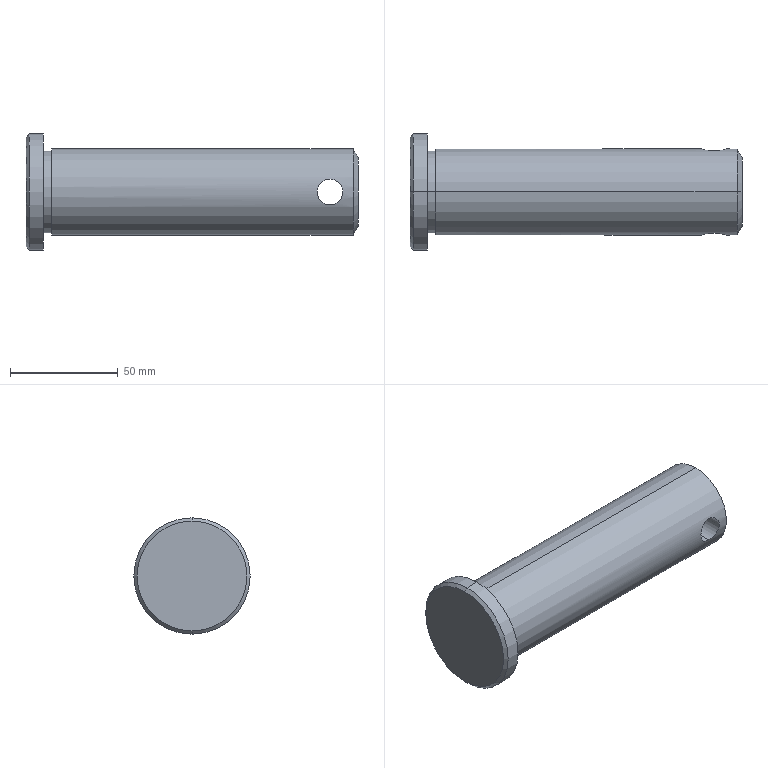Part | SolidWorks | features Chamfer 2, ICE 1, Revolution 1 | 1 solid | 16 faces | box 154 x 54 x 54 mm | volume 196099 mm3 | cylinder 8 | cone 4 | plane 4 | commonest cylinder face diameters 12 x2 38 x2 40 x2 54 x2
STEP:
#1=CARTESIAN_POINT('',(141.,-19.079,-6.));
#2=VERTEX_POINT('',#1);
#3=CARTESIAN_POINT('',(141.,-19.079,6.));
#4=VERTEX_POINT('',#3);
#5=CARTESIAN_POINT('',(141.,-19.079,-6.));
#6=CARTESIAN_POINT('',(140.607,-19.079,-6.));
#7=CARTESIAN_POINT('',(140.213,-19.091,-5.961));
#8=CARTESIAN_POINT('',(139.434,-19.139,-5.806));
#9=CARTESIAN_POINT('',(139.059,-19.174,-5.691));
#10=CARTESIAN_POINT('',(138.336,-19.261,-5.39));
#11=CARTESIAN_POINT('',(137.985,-19.313,-5.202));
#12=CARTESIAN_POINT('',(137.336,-19.425,-4.767));
#13=CARTESIAN_POINT('',(137.035,-19.484,-4.521));
#14=CARTESIAN_POINT('',(136.62,-19.575,-4.105));
#15=CARTESIAN_POINT('',(136.487,-19.605,-3.959));
#16=CARTESIAN_POINT('',(136.239,-19.664,-3.657));
#17=CARTESIAN_POINT('',(136.123,-19.692,-3.5));
#18=CARTESIAN_POINT('',(135.798,-19.774,-3.015));
#19=CARTESIAN_POINT('',(135.612,-19.824,-2.67));
#20=CARTESIAN_POINT('',(135.308,-19.909,-1.939));
#21=CARTESIAN_POINT('',(135.194,-19.943,-1.564));
#22=CARTESIAN_POINT('',(135.078,-19.977,-0.9868));
#23=CARTESIAN_POINT('',(135.049,-19.985,-0.7922));
#24=CARTESIAN_POINT('',(135.01,-19.997,-0.398));
#25=CARTESIAN_POINT('',(135.,-20.,-0.1981));
#26=CARTESIAN_POINT('',(135.,-20.,0.3951));
#27=CARTESIAN_POINT('',(135.039,-19.988,0.7861));
#28=CARTESIAN_POINT('',(135.154,-19.954,1.366));
#29=CARTESIAN_POINT('',(135.203,-19.94,1.559));
#30=CARTESIAN_POINT('',(135.318,-19.907,1.938));
#31=CARTESIAN_POINT('',(135.385,-19.888,2.123));
#32=CARTESIAN_POINT('',(135.61,-19.825,2.665));
#33=CARTESIAN_POINT('',(135.795,-19.775,3.01));
#34=CARTESIAN_POINT('',(136.234,-19.664,3.666));
#35=CARTESIAN_POINT('',(136.481,-19.605,3.967));
#36=CARTESIAN_POINT('',(136.894,-19.515,4.379));
#37=CARTESIAN_POINT('',(137.038,-19.485,4.51));
#38=CARTESIAN_POINT('',(137.341,-19.426,4.759));
#39=CARTESIAN_POINT('',(137.5,-19.397,4.877));
#40=CARTESIAN_POINT('',(137.988,-19.312,5.204));
#41=CARTESIAN_POINT('',(138.331,-19.261,5.388));
#42=CARTESIAN_POINT('',(139.054,-19.174,5.689));
#43=CARTESIAN_POINT('',(139.437,-19.139,5.806));
#44=CARTESIAN_POINT('',(140.209,-19.091,5.961));
#45=CARTESIAN_POINT('',(140.601,-19.079,6.));
#46=CARTESIAN_POINT('',(141.,-19.079,6.));
#47=B_SPLINE_CURVE_WITH_KNOTS('',3,(#5,#6,#7,#8,#9,#10,#11,#12,#13,#14,#15,#16,#17,#18,#19,#20,#21,#22,#23,#24,#25,#26,#27,#28,#29,#30,#31,#32,#33,#34,#35,#36,#37,#38,#39,#40,#41,#42,#43,#44,#45,#46),.UNSPECIFIED.,.F.,.F.,(4,2,2,2,2,2,2,2,2,2,2,2,2,2,2,2,2,2,2,2,4),(0.01887,0.02005,0.02123,0.0224,0.02358,0.02417,0.02476,0.02594,0.02712,0.02771,0.0283,0.02948,0.03007,0.03066,0.03184,0.03301,0.0336,0.03419,0.03537,0.03655,0.03773),.UNSPECIFIED.);
#48=EDGE_CURVE('',#2,#4,#47,.T.);
#49=ORIENTED_EDGE('',*,*,#48,.F.);
#50=CARTESIAN_POINT('',(141.,19.079,-6.));
#51=VERTEX_POINT('',#50);
#52=CARTESIAN_POINT('',(141.,-27.,-6.));
#53=DIRECTION('',(0.,1.,0.));
#54=VECTOR('',#53,1000.);
#55=LINE('',#52,#54);
#56=EDGE_CURVE('',#2,#51,#55,.T.);
#57=ORIENTED_EDGE('',*,*,#56,.T.);
#58=CARTESIAN_POINT('',(141.,19.079,6.));
#59=VERTEX_POINT('',#58);
#60=CARTESIAN_POINT('',(141.,19.079,6.));
#61=CARTESIAN_POINT('',(140.601,19.079,6.));
#62=CARTESIAN_POINT('',(140.209,19.091,5.961));
#63=CARTESIAN_POINT('',(139.632,19.127,5.845));
#64=CARTESIAN_POINT('',(139.441,19.141,5.797));
#65=CARTESIAN_POINT('',(139.063,19.176,5.682));
#66=CARTESIAN_POINT('',(138.876,19.196,5.615));
#67=CARTESIAN_POINT('',(138.332,19.261,5.388));
#68=CARTESIAN_POINT('',(137.988,19.312,5.204));
#69=CARTESIAN_POINT('',(137.5,19.396,4.877));
#70=CARTESIAN_POINT('',(137.341,19.426,4.759));
#71=CARTESIAN_POINT('',(137.038,19.485,4.51));
#72=CARTESIAN_POINT('',(136.894,19.515,4.379));
#73=CARTESIAN_POINT('',(136.482,19.605,3.967));
#74=CARTESIAN_POINT('',(136.234,19.664,3.666));
#75=CARTESIAN_POINT('',(135.795,19.775,3.011));
#76=CARTESIAN_POINT('',(135.61,19.825,2.665));
#77=CARTESIAN_POINT('',(135.385,19.888,2.124));
#78=CARTESIAN_POINT('',(135.319,19.907,1.94));
#79=CARTESIAN_POINT('',(135.204,19.94,1.563));
#80=CARTESIAN_POINT('',(135.155,19.954,1.369));
#81=CARTESIAN_POINT('',(135.039,19.988,0.7875));
#82=CARTESIAN_POINT('',(135.,20.,0.3966));
#83=CARTESIAN_POINT('',(135.,20.,-0.3914));
#84=CARTESIAN_POINT('',(135.039,19.988,-0.7916));
#85=CARTESIAN_POINT('',(135.194,19.943,-1.563));
#86=CARTESIAN_POINT('',(135.308,19.909,-1.938));
#87=CARTESIAN_POINT('',(135.611,19.825,-2.668));
#88=CARTESIAN_POINT('',(135.798,19.774,-3.015));
#89=CARTESIAN_POINT('',(136.123,19.692,-3.501));
#90=CARTESIAN_POINT('',(136.24,19.663,-3.657));
#91=CARTESIAN_POINT('',(136.488,19.605,-3.96));
#92=CARTESIAN_POINT('',(136.621,19.574,-4.106));
#93=CARTESIAN_POINT('',(137.037,19.484,-4.522));
#94=CARTESIAN_POINT('',(137.337,19.425,-4.768));
#95=CARTESIAN_POINT('',(137.985,19.313,-5.202));
#96=CARTESIAN_POINT('',(138.337,19.26,-5.391));
#97=CARTESIAN_POINT('',(139.06,19.174,-5.691));
#98=CARTESIAN_POINT('',(139.434,19.139,-5.805));
#99=CARTESIAN_POINT('',(140.015,19.103,-5.922));
#100=CARTESIAN_POINT('',(140.213,19.094,-5.951));
#101=CARTESIAN_POINT('',(140.607,19.082,-5.99));
#102=CARTESIAN_POINT('',(140.803,19.079,-6.));
#103=CARTESIAN_POINT('',(141.,19.079,-6.));
#104=B_SPLINE_CURVE_WITH_KNOTS('',3,(#60,#61,#62,#63,#64,#65,#66,#67,#68,#69,#70,#71,#72,#73,#74,#75,#76,#77,#78,#79,#80,#81,#82,#83,#84,#85,#86,#87,#88,#89,#90,#91,#92,#93,#94,#95,#96,#97,#98,#99,#100,#101,#102,#103),.UNSPECIFIED.,.F.,.F.,(4,2,2,2,2,2,2,2,2,2,2,2,2,2,2,2,2,2,2,2,2,4),(0.,0.001179,0.001769,0.002358,0.003538,0.004127,0.004717,0.005896,0.007075,0.007665,0.008255,0.009434,0.01061,0.01179,0.01297,0.01356,0.01415,0.01533,0.01651,0.01769,0.01828,0.01887),.UNSPECIFIED.);
#105=EDGE_CURVE('',#59,#51,#104,.T.);
#106=ORIENTED_EDGE('',*,*,#105,.F.);
#107=CARTESIAN_POINT('',(141.,-27.,6.));
#108=DIRECTION('',(0.,1.,0.));
#109=VECTOR('',#108,1000.);
#110=LINE('',#107,#109);
#111=EDGE_CURVE('',#4,#59,#110,.T.);
#112=ORIENTED_EDGE('',*,*,#111,.F.);
#113=EDGE_LOOP('',(#49,#57,#106,#112));
#114=FACE_OUTER_BOUND('',#113,.T.);
#115=CARTESIAN_POINT('',(141.,-27.,0.));
#116=DIRECTION('',(0.,1.,0.));
#117=DIRECTION('',(0.,0.,1.));
#118=AXIS2_PLACEMENT_3D('',#115,#116,#117);
#119=CYLINDRICAL_SURFACE('',#118,6.);
#120=ADVANCED_FACE('',(#114),#119,.F.);
#121=CARTESIAN_POINT('',(154.,0.,-16.));
#122=VERTEX_POINT('',#121);
#123=CARTESIAN_POINT('',(154.,0.,16.));
#124=VERTEX_POINT('',#123);
#125=CARTESIAN_POINT('',(154.,0.,0.));
#126=DIRECTION('',(1.,0.,0.));
#127=DIRECTION('',(0.,0.,1.));
#128=AXIS2_PLACEMENT_3D('',#125,#126,#127);
#129=CIRCLE('',#128,16.);
#130=EDGE_CURVE('',#122,#124,#129,.T.);
#131=ORIENTED_EDGE('',*,*,#130,.F.);
#132=CARTESIAN_POINT('',(151.691,0.,-20.));
#133=VERTEX_POINT('',#132);
#134=CARTESIAN_POINT('',(151.691,0.,-20.));
#135=DIRECTION('',(-0.5,0.,-0.866));
#136=VECTOR('',#135,1000.);
#137=LINE('',#134,#136);
#138=EDGE_CURVE('',#122,#133,#137,.T.);
#139=ORIENTED_EDGE('',*,*,#138,.T.);
#140=CARTESIAN_POINT('',(151.691,0.,20.));
#141=VERTEX_POINT('',#140);
#142=CARTESIAN_POINT('',(151.691,0.,0.));
#143=DIRECTION('',(-1.,0.,0.));
#144=DIRECTION('',(0.,0.,1.));
#145=AXIS2_PLACEMENT_3D('',#142,#143,#144);
#146=CIRCLE('',#145,20.);
#147=EDGE_CURVE('',#141,#133,#146,.T.);
#148=ORIENTED_EDGE('',*,*,#147,.F.);
#149=CARTESIAN_POINT('',(151.691,0.,20.));
#150=DIRECTION('',(-0.5,0.,0.866));
#151=VECTOR('',#150,1000.);
#152=LINE('',#149,#151);
#153=EDGE_CURVE('',#124,#141,#152,.T.);
#154=ORIENTED_EDGE('',*,*,#153,.F.);
#155=EDGE_LOOP('',(#131,#139,#148,#154));
#156=FACE_OUTER_BOUND('',#155,.T.);
#157=CARTESIAN_POINT('',(151.691,0.,0.));
#158=DIRECTION('',(-1.,0.,0.));
#159=DIRECTION('',(0.,0.,1.));
#160=AXIS2_PLACEMENT_3D('',#157,#158,#159);
#161=CONICAL_SURFACE('',#160,20.,1.047);
#162=ADVANCED_FACE('',(#156),#161,.T.);
#163=CARTESIAN_POINT('',(0.,0.,25.5));
#164=VERTEX_POINT('',#163);
#165=CARTESIAN_POINT('',(0.,0.,-25.5));
#166=VERTEX_POINT('',#165);
#167=CARTESIAN_POINT('',(0.,0.,0.));
#168=DIRECTION('',(-1.,0.,0.));
#169=DIRECTION('',(0.,0.,-1.));
#170=AXIS2_PLACEMENT_3D('',#167,#168,#169);
#171=CIRCLE('',#170,25.5);
#172=EDGE_CURVE('',#164,#166,#171,.T.);
#173=ORIENTED_EDGE('',*,*,#172,.F.);
#174=CARTESIAN_POINT('',(1.5,0.,27.));
#175=VERTEX_POINT('',#174);
#176=CARTESIAN_POINT('',(0.,0.,25.5));
#177=DIRECTION('',(0.7071,0.,0.7071));
#178=VECTOR('',#177,1000.);
#179=LINE('',#176,#178);
#180=EDGE_CURVE('',#164,#175,#179,.T.);
#181=ORIENTED_EDGE('',*,*,#180,.T.);
#182=CARTESIAN_POINT('',(1.5,0.,-27.));
#183=VERTEX_POINT('',#182);
#184=CARTESIAN_POINT('',(1.5,0.,0.));
#185=DIRECTION('',(1.,0.,0.));
#186=DIRECTION('',(0.,0.,-1.));
#187=AXIS2_PLACEMENT_3D('',#184,#185,#186);
#188=CIRCLE('',#187,27.);
#189=EDGE_CURVE('',#183,#175,#188,.T.);
#190=ORIENTED_EDGE('',*,*,#189,.F.);
#191=CARTESIAN_POINT('',(0.,0.,-25.5));
#192=DIRECTION('',(0.7071,0.,-0.7071));
#193=VECTOR('',#192,1000.);
#194=LINE('',#191,#193);
#195=EDGE_CURVE('',#166,#183,#194,.T.);
#196=ORIENTED_EDGE('',*,*,#195,.F.);
#197=EDGE_LOOP('',(#173,#181,#190,#196));
#198=FACE_OUTER_BOUND('',#197,.T.);
#199=CARTESIAN_POINT('',(0.,0.,0.));
#200=DIRECTION('',(1.,0.,0.));
#201=DIRECTION('',(0.,0.,-1.));
#202=AXIS2_PLACEMENT_3D('',#199,#200,#201);
#203=CONICAL_SURFACE('',#202,25.5,0.7854);
#204=ADVANCED_FACE('',(#198),#203,.T.);
#205=CARTESIAN_POINT('',(8.,0.,27.));
#206=VERTEX_POINT('',#205);
#207=CARTESIAN_POINT('',(8.,0.,-27.));
#208=VERTEX_POINT('',#207);
#209=CARTESIAN_POINT('',(8.,0.,0.));
#210=DIRECTION('',(-1.,0.,0.));
#211=DIRECTION('',(0.,0.,1.));
#212=AXIS2_PLACEMENT_3D('',#209,#210,#211);
#213=CIRCLE('',#212,27.);
#214=EDGE_CURVE('',#206,#208,#213,.T.);
#215=ORIENTED_EDGE('',*,*,#214,.T.);
#216=CARTESIAN_POINT('',(-105.652,0.,-27.));
#217=DIRECTION('',(-1.,0.,0.));
#218=VECTOR('',#217,1000.);
#219=LINE('',#216,#218);
#220=EDGE_CURVE('',#208,#183,#219,.T.);
#221=ORIENTED_EDGE('',*,*,#220,.T.);
#222=ORIENTED_EDGE('',*,*,#189,.T.);
#223=CARTESIAN_POINT('',(-105.652,0.,27.));
#224=DIRECTION('',(-1.,0.,0.));
#225=VECTOR('',#224,1000.);
#226=LINE('',#223,#225);
#227=EDGE_CURVE('',#206,#175,#226,.T.);
#228=ORIENTED_EDGE('',*,*,#227,.F.);
#229=EDGE_LOOP('',(#215,#221,#222,#228));
#230=FACE_OUTER_BOUND('',#229,.T.);
#231=CARTESIAN_POINT('',(-105.652,0.,0.));
#232=DIRECTION('',(-1.,0.,0.));
#233=DIRECTION('',(0.,0.,1.));
#234=AXIS2_PLACEMENT_3D('',#231,#232,#233);
#235=CYLINDRICAL_SURFACE('',#234,27.);
#236=ADVANCED_FACE('',(#230),#235,.T.);
#237=CARTESIAN_POINT('',(12.,0.,19.));
#238=VERTEX_POINT('',#237);
#239=CARTESIAN_POINT('',(12.,0.,-19.));
#240=VERTEX_POINT('',#239);
#241=CARTESIAN_POINT('',(12.,0.,0.));
#242=DIRECTION('',(-1.,0.,0.));
#243=DIRECTION('',(0.,0.,1.));
#244=AXIS2_PLACEMENT_3D('',#241,#242,#243);
#245=CIRCLE('',#244,19.);
#246=EDGE_CURVE('',#238,#240,#245,.T.);
#247=ORIENTED_EDGE('',*,*,#246,.T.);
#248=CARTESIAN_POINT('',(8.,0.,-19.));
#249=VERTEX_POINT('',#248);
#250=CARTESIAN_POINT('',(-105.652,0.,-19.));
#251=DIRECTION('',(-1.,0.,0.));
#252=VECTOR('',#251,1000.);
#253=LINE('',#250,#252);
#254=EDGE_CURVE('',#240,#249,#253,.T.);
#255=ORIENTED_EDGE('',*,*,#254,.T.);
#256=CARTESIAN_POINT('',(8.,0.,19.));
#257=VERTEX_POINT('',#256);
#258=CARTESIAN_POINT('',(8.,0.,0.));
#259=DIRECTION('',(-1.,0.,0.));
#260=DIRECTION('',(0.,0.,1.));
#261=AXIS2_PLACEMENT_3D('',#258,#259,#260);
#262=CIRCLE('',#261,19.);
#263=EDGE_CURVE('',#257,#249,#262,.T.);
#264=ORIENTED_EDGE('',*,*,#263,.F.);
#265=CARTESIAN_POINT('',(-105.652,0.,19.));
#266=DIRECTION('',(-1.,0.,0.));
#267=VECTOR('',#266,1000.);
#268=LINE('',#265,#267);
#269=EDGE_CURVE('',#238,#257,#268,.T.);
#270=ORIENTED_EDGE('',*,*,#269,.F.);
#271=EDGE_LOOP('',(#247,#255,#264,#270));
#272=FACE_OUTER_BOUND('',#271,.T.);
#273=CARTESIAN_POINT('',(-105.652,0.,0.));
#274=DIRECTION('',(-1.,0.,0.));
#275=DIRECTION('',(0.,0.,1.));
#276=AXIS2_PLACEMENT_3D('',#273,#274,#275);
#277=CYLINDRICAL_SURFACE('',#276,19.);
#278=ADVANCED_FACE('',(#272),#277,.T.);
#279=ORIENTED_EDGE('',*,*,#105,.T.);
#280=CARTESIAN_POINT('',(141.,19.079,-6.));
#281=CARTESIAN_POINT('',(141.393,19.079,-6.));
#282=CARTESIAN_POINT('',(141.787,19.091,-5.961));
#283=CARTESIAN_POINT('',(142.566,19.139,-5.806));
#284=CARTESIAN_POINT('',(142.941,19.174,-5.691));
#285=CARTESIAN_POINT('',(143.664,19.261,-5.39));
#286=CARTESIAN_POINT('',(144.015,19.313,-5.202));
#287=CARTESIAN_POINT('',(144.664,19.425,-4.767));
#288=CARTESIAN_POINT('',(144.965,19.484,-4.521));
#289=CARTESIAN_POINT('',(145.38,19.575,-4.105));
#290=CARTESIAN_POINT('',(145.513,19.605,-3.959));
#291=CARTESIAN_POINT('',(145.761,19.664,-3.657));
#292=CARTESIAN_POINT('',(145.877,19.692,-3.5));
#293=CARTESIAN_POINT('',(146.202,19.774,-3.015));
#294=CARTESIAN_POINT('',(146.388,19.824,-2.67));
#295=CARTESIAN_POINT('',(146.692,19.909,-1.939));
#296=CARTESIAN_POINT('',(146.806,19.943,-1.564));
#297=CARTESIAN_POINT('',(146.922,19.977,-0.9868));
#298=CARTESIAN_POINT('',(146.951,19.985,-0.7922));
#299=CARTESIAN_POINT('',(146.99,19.997,-0.398));
#300=CARTESIAN_POINT('',(147.,20.,-0.1981));
#301=CARTESIAN_POINT('',(147.,20.,0.3951));
#302=CARTESIAN_POINT('',(146.961,19.988,0.7861));
#303=CARTESIAN_POINT('',(146.846,19.954,1.366));
#304=CARTESIAN_POINT('',(146.797,19.94,1.559));
#305=CARTESIAN_POINT('',(146.682,19.907,1.938));
#306=CARTESIAN_POINT('',(146.615,19.888,2.123));
#307=CARTESIAN_POINT('',(146.39,19.825,2.665));
#308=CARTESIAN_POINT('',(146.205,19.775,3.01));
#309=CARTESIAN_POINT('',(145.766,19.664,3.666));
#310=CARTESIAN_POINT('',(145.519,19.605,3.967));
#311=CARTESIAN_POINT('',(145.106,19.515,4.379));
#312=CARTESIAN_POINT('',(144.962,19.485,4.51));
#313=CARTESIAN_POINT('',(144.659,19.426,4.759));
#314=CARTESIAN_POINT('',(144.5,19.397,4.877));
#315=CARTESIAN_POINT('',(144.012,19.312,5.204));
#316=CARTESIAN_POINT('',(143.669,19.261,5.388));
#317=CARTESIAN_POINT('',(142.946,19.174,5.689));
#318=CARTESIAN_POINT('',(142.563,19.139,5.806));
#319=CARTESIAN_POINT('',(141.791,19.091,5.961));
#320=CARTESIAN_POINT('',(141.399,19.079,6.));
#321=CARTESIAN_POINT('',(141.,19.079,6.));
#322=B_SPLINE_CURVE_WITH_KNOTS('',3,(#280,#281,#282,#283,#284,#285,#286,#287,#288,#289,#290,#291,#292,#293,#294,#295,#296,#297,#298,#299,#300,#301,#302,#303,#304,#305,#306,#307,#308,#309,#310,#311,#312,#313,#314,#315,#316,#317,#318,#319,#320,#321),.UNSPECIFIED.,.F.,.F.,(4,2,2,2,2,2,2,2,2,2,2,2,2,2,2,2,2,2,2,2,4),(0.01887,0.02005,0.02123,0.0224,0.02358,0.02417,0.02476,0.02594,0.02712,0.02771,0.0283,0.02948,0.03007,0.03066,0.03184,0.03301,0.0336,0.03419,0.03537,0.03655,0.03773),.UNSPECIFIED.);
#323=EDGE_CURVE('',#51,#59,#322,.T.);
#324=ORIENTED_EDGE('',*,*,#323,.T.);
#325=EDGE_LOOP('',(#279,#324));
#326=FACE_BOUND('',#325,.T.);
#327=ORIENTED_EDGE('',*,*,#147,.T.);
#328=CARTESIAN_POINT('',(12.,0.,-20.));
#329=VERTEX_POINT('',#328);
#330=CARTESIAN_POINT('',(-105.652,0.,-20.));
#331=DIRECTION('',(-1.,0.,0.));
#332=VECTOR('',#331,1000.);
#333=LINE('',#330,#332);
#334=EDGE_CURVE('',#133,#329,#333,.T.);
#335=ORIENTED_EDGE('',*,*,#334,.T.);
#336=CARTESIAN_POINT('',(12.,0.,20.));
#337=VERTEX_POINT('',#336);
#338=CARTESIAN_POINT('',(12.,0.,0.));
#339=DIRECTION('',(-1.,0.,0.));
#340=DIRECTION('',(0.,0.,1.));
#341=AXIS2_PLACEMENT_3D('',#338,#339,#340);
#342=CIRCLE('',#341,20.);
#343=EDGE_CURVE('',#337,#329,#342,.T.);
#344=ORIENTED_EDGE('',*,*,#343,.F.);
#345=CARTESIAN_POINT('',(-105.652,0.,20.));
#346=DIRECTION('',(-1.,0.,0.));
#347=VECTOR('',#346,1000.);
#348=LINE('',#345,#347);
#349=EDGE_CURVE('',#141,#337,#348,.T.);
#350=ORIENTED_EDGE('',*,*,#349,.F.);
#351=EDGE_LOOP('',(#327,#335,#344,#350));
#352=FACE_OUTER_BOUND('',#351,.T.);
#353=CARTESIAN_POINT('',(-105.652,0.,0.));
#354=DIRECTION('',(-1.,0.,0.));
#355=DIRECTION('',(0.,0.,1.));
#356=AXIS2_PLACEMENT_3D('',#353,#354,#355);
#357=CYLINDRICAL_SURFACE('',#356,20.);
#358=ADVANCED_FACE('',(#326,#352),#357,.T.);
#359=CARTESIAN_POINT('',(0.,0.,0.));
#360=DIRECTION('',(-1.,0.,0.));
#361=DIRECTION('',(0.,0.,-1.));
#362=AXIS2_PLACEMENT_3D('',#359,#360,#361);
#363=CIRCLE('',#362,25.5);
#364=EDGE_CURVE('',#166,#164,#363,.T.);
#365=ORIENTED_EDGE('',*,*,#364,.T.);
#366=ORIENTED_EDGE('',*,*,#172,.T.);
#367=EDGE_LOOP('',(#365,#366));
#368=FACE_OUTER_BOUND('',#367,.T.);
#369=CARTESIAN_POINT('',(0.,27.,0.));
#370=DIRECTION('',(1.,0.,0.));
#371=DIRECTION('',(0.,0.,-1.));
#372=AXIS2_PLACEMENT_3D('',#369,#370,#371);
#373=PLANE('',#372);
#374=ADVANCED_FACE('',(#368),#373,.F.);
#375=CARTESIAN_POINT('',(154.,0.,0.));
#376=DIRECTION('',(1.,0.,0.));
#377=DIRECTION('',(0.,0.,1.));
#378=AXIS2_PLACEMENT_3D('',#375,#376,#377);
#379=CIRCLE('',#378,16.);
#380=EDGE_CURVE('',#124,#122,#379,.T.);
#381=ORIENTED_EDGE('',*,*,#380,.T.);
#382=ORIENTED_EDGE('',*,*,#130,.T.);
#383=EDGE_LOOP('',(#381,#382));
#384=FACE_OUTER_BOUND('',#383,.T.);
#385=CARTESIAN_POINT('',(154.,0.,0.));
#386=DIRECTION('',(-1.,0.,0.));
#387=DIRECTION('',(0.,0.,1.));
#388=AXIS2_PLACEMENT_3D('',#385,#386,#387);
#389=PLANE('',#388);
#390=ADVANCED_FACE('',(#384),#389,.F.);
#391=ORIENTED_EDGE('',*,*,#334,.F.);
#392=CARTESIAN_POINT('',(151.691,0.,0.));
#393=DIRECTION('',(-1.,0.,0.));
#394=DIRECTION('',(0.,0.,1.));
#395=AXIS2_PLACEMENT_3D('',#392,#393,#394);
#396=CIRCLE('',#395,20.);
#397=EDGE_CURVE('',#133,#141,#396,.T.);
#398=ORIENTED_EDGE('',*,*,#397,.T.);
#399=ORIENTED_EDGE('',*,*,#349,.T.);
#400=CARTESIAN_POINT('',(12.,0.,0.));
#401=DIRECTION('',(-1.,0.,0.));
#402=DIRECTION('',(0.,0.,1.));
#403=AXIS2_PLACEMENT_3D('',#400,#401,#402);
#404=CIRCLE('',#403,20.);
#405=EDGE_CURVE('',#329,#337,#404,.T.);
#406=ORIENTED_EDGE('',*,*,#405,.F.);
#407=EDGE_LOOP('',(#391,#398,#399,#406));
#408=FACE_OUTER_BOUND('',#407,.T.);
#409=CARTESIAN_POINT('',(141.,-19.079,6.));
#410=CARTESIAN_POINT('',(141.399,-19.079,6.));
#411=CARTESIAN_POINT('',(141.791,-19.091,5.961));
#412=CARTESIAN_POINT('',(142.368,-19.127,5.845));
#413=CARTESIAN_POINT('',(142.559,-19.141,5.797));
#414=CARTESIAN_POINT('',(142.937,-19.176,5.682));
#415=CARTESIAN_POINT('',(143.124,-19.196,5.615));
#416=CARTESIAN_POINT('',(143.668,-19.261,5.388));
#417=CARTESIAN_POINT('',(144.012,-19.312,5.204));
#418=CARTESIAN_POINT('',(144.5,-19.396,4.877));
#419=CARTESIAN_POINT('',(144.659,-19.426,4.759));
#420=CARTESIAN_POINT('',(144.962,-19.485,4.51));
#421=CARTESIAN_POINT('',(145.106,-19.515,4.379));
#422=CARTESIAN_POINT('',(145.518,-19.605,3.967));
#423=CARTESIAN_POINT('',(145.766,-19.664,3.666));
#424=CARTESIAN_POINT('',(146.205,-19.775,3.011));
#425=CARTESIAN_POINT('',(146.39,-19.825,2.665));
#426=CARTESIAN_POINT('',(146.615,-19.888,2.124));
#427=CARTESIAN_POINT('',(146.681,-19.907,1.94));
#428=CARTESIAN_POINT('',(146.796,-19.94,1.563));
#429=CARTESIAN_POINT('',(146.845,-19.954,1.369));
#430=CARTESIAN_POINT('',(146.961,-19.988,0.7875));
#431=CARTESIAN_POINT('',(147.,-20.,0.3966));
#432=CARTESIAN_POINT('',(147.,-20.,-0.3914));
#433=CARTESIAN_POINT('',(146.961,-19.988,-0.7916));
#434=CARTESIAN_POINT('',(146.806,-19.943,-1.563));
#435=CARTESIAN_POINT('',(146.692,-19.909,-1.938));
#436=CARTESIAN_POINT('',(146.389,-19.825,-2.668));
#437=CARTESIAN_POINT('',(146.202,-19.774,-3.015));
#438=CARTESIAN_POINT('',(145.877,-19.692,-3.501));
#439=CARTESIAN_POINT('',(145.76,-19.663,-3.657));
#440=CARTESIAN_POINT('',(145.512,-19.605,-3.96));
#441=CARTESIAN_POINT('',(145.379,-19.574,-4.106));
#442=CARTESIAN_POINT('',(144.963,-19.484,-4.522));
#443=CARTESIAN_POINT('',(144.663,-19.425,-4.768));
#444=CARTESIAN_POINT('',(144.015,-19.313,-5.202));
#445=CARTESIAN_POINT('',(143.663,-19.26,-5.391));
#446=CARTESIAN_POINT('',(142.94,-19.174,-5.691));
#447=CARTESIAN_POINT('',(142.566,-19.139,-5.805));
#448=CARTESIAN_POINT('',(141.985,-19.103,-5.922));
#449=CARTESIAN_POINT('',(141.787,-19.094,-5.951));
#450=CARTESIAN_POINT('',(141.393,-19.082,-5.99));
#451=CARTESIAN_POINT('',(141.197,-19.079,-6.));
#452=CARTESIAN_POINT('',(141.,-19.079,-6.));
#453=B_SPLINE_CURVE_WITH_KNOTS('',3,(#409,#410,#411,#412,#413,#414,#415,#416,#417,#418,#419,#420,#421,#422,#423,#424,#425,#426,#427,#428,#429,#430,#431,#432,#433,#434,#435,#436,#437,#438,#439,#440,#441,#442,#443,#444,#445,#446,#447,#448,#449,#450,#451,#452),.UNSPECIFIED.,.F.,.F.,(4,2,2,2,2,2,2,2,2,2,2,2,2,2,2,2,2,2,2,2,2,4),(0.,0.001179,0.001769,0.002358,0.003538,0.004127,0.004717,0.005896,0.007075,0.007665,0.008255,0.009434,0.01061,0.01179,0.01297,0.01356,0.01415,0.01533,0.01651,0.01769,0.01828,0.01887),.UNSPECIFIED.);
#454=EDGE_CURVE('',#4,#2,#453,.T.);
#455=ORIENTED_EDGE('',*,*,#454,.T.);
#456=ORIENTED_EDGE('',*,*,#48,.T.);
#457=EDGE_LOOP('',(#455,#456));
#458=FACE_BOUND('',#457,.T.);
#459=CARTESIAN_POINT('',(-105.652,0.,0.));
#460=DIRECTION('',(-1.,0.,0.));
#461=DIRECTION('',(0.,0.,1.));
#462=AXIS2_PLACEMENT_3D('',#459,#460,#461);
#463=CYLINDRICAL_SURFACE('',#462,20.);
#464=ADVANCED_FACE('',(#408,#458),#463,.T.);
#465=ORIENTED_EDGE('',*,*,#246,.F.);
#466=CARTESIAN_POINT('',(12.,0.,0.));
#467=DIRECTION('',(-1.,0.,0.));
#468=DIRECTION('',(0.,0.,1.));
#469=AXIS2_PLACEMENT_3D('',#466,#467,#468);
#470=CIRCLE('',#469,19.);
#471=EDGE_CURVE('',#240,#238,#470,.T.);
#472=ORIENTED_EDGE('',*,*,#471,.F.);
#473=EDGE_LOOP('',(#465,#472));
#474=FACE_BOUND('',#473,.T.);
#475=ORIENTED_EDGE('',*,*,#343,.T.);
#476=ORIENTED_EDGE('',*,*,#405,.T.);
#477=EDGE_LOOP('',(#475,#476));
#478=FACE_OUTER_BOUND('',#477,.T.);
#479=CARTESIAN_POINT('',(12.,20.,0.));
#480=DIRECTION('',(1.,0.,0.));
#481=DIRECTION('',(0.,0.,-1.));
#482=AXIS2_PLACEMENT_3D('',#479,#480,#481);
#483=PLANE('',#482);
#484=ADVANCED_FACE('',(#474,#478),#483,.F.);
#485=ORIENTED_EDGE('',*,*,#254,.F.);
#486=ORIENTED_EDGE('',*,*,#471,.T.);
#487=ORIENTED_EDGE('',*,*,#269,.T.);
#488=CARTESIAN_POINT('',(8.,0.,0.));
#489=DIRECTION('',(-1.,0.,0.));
#490=DIRECTION('',(0.,0.,1.));
#491=AXIS2_PLACEMENT_3D('',#488,#489,#490);
#492=CIRCLE('',#491,19.);
#493=EDGE_CURVE('',#249,#257,#492,.T.);
#494=ORIENTED_EDGE('',*,*,#493,.F.);
#495=EDGE_LOOP('',(#485,#486,#487,#494));
#496=FACE_OUTER_BOUND('',#495,.T.);
#497=CARTESIAN_POINT('',(-105.652,0.,0.));
#498=DIRECTION('',(-1.,0.,0.));
#499=DIRECTION('',(0.,0.,1.));
#500=AXIS2_PLACEMENT_3D('',#497,#498,#499);
#501=CYLINDRICAL_SURFACE('',#500,19.);
#502=ADVANCED_FACE('',(#496),#501,.T.);
#503=ORIENTED_EDGE('',*,*,#214,.F.);
#504=CARTESIAN_POINT('',(8.,0.,0.));
#505=DIRECTION('',(-1.,0.,0.));
#506=DIRECTION('',(0.,0.,1.));
#507=AXIS2_PLACEMENT_3D('',#504,#505,#506);
#508=CIRCLE('',#507,27.);
#509=EDGE_CURVE('',#208,#206,#508,.T.);
#510=ORIENTED_EDGE('',*,*,#509,.F.);
#511=EDGE_LOOP('',(#503,#510));
#512=FACE_OUTER_BOUND('',#511,.T.);
#513=ORIENTED_EDGE('',*,*,#263,.T.);
#514=ORIENTED_EDGE('',*,*,#493,.T.);
#515=EDGE_LOOP('',(#513,#514));
#516=FACE_BOUND('',#515,.T.);
#517=CARTESIAN_POINT('',(8.,19.,0.));
#518=DIRECTION('',(-1.,0.,0.));
#519=DIRECTION('',(0.,0.,1.));
#520=AXIS2_PLACEMENT_3D('',#517,#518,#519);
#521=PLANE('',#520);
#522=ADVANCED_FACE('',(#512,#516),#521,.F.);
#523=ORIENTED_EDGE('',*,*,#220,.F.);
#524=ORIENTED_EDGE('',*,*,#509,.T.);
#525=ORIENTED_EDGE('',*,*,#227,.T.);
#526=CARTESIAN_POINT('',(1.5,0.,0.));
#527=DIRECTION('',(1.,0.,0.));
#528=DIRECTION('',(0.,0.,-1.));
#529=AXIS2_PLACEMENT_3D('',#526,#527,#528);
#530=CIRCLE('',#529,27.);
#531=EDGE_CURVE('',#175,#183,#530,.T.);
#532=ORIENTED_EDGE('',*,*,#531,.T.);
#533=EDGE_LOOP('',(#523,#524,#525,#532));
#534=FACE_OUTER_BOUND('',#533,.T.);
#535=CARTESIAN_POINT('',(-105.652,0.,0.));
#536=DIRECTION('',(-1.,0.,0.));
#537=DIRECTION('',(0.,0.,1.));
#538=AXIS2_PLACEMENT_3D('',#535,#536,#537);
#539=CYLINDRICAL_SURFACE('',#538,27.);
#540=ADVANCED_FACE('',(#534),#539,.T.);
#541=ORIENTED_EDGE('',*,*,#180,.F.);
#542=ORIENTED_EDGE('',*,*,#364,.F.);
#543=ORIENTED_EDGE('',*,*,#195,.T.);
#544=ORIENTED_EDGE('',*,*,#531,.F.);
#545=EDGE_LOOP('',(#541,#542,#543,#544));
#546=FACE_OUTER_BOUND('',#545,.T.);
#547=CARTESIAN_POINT('',(0.,0.,0.));
#548=DIRECTION('',(1.,0.,0.));
#549=DIRECTION('',(0.,0.,-1.));
#550=AXIS2_PLACEMENT_3D('',#547,#548,#549);
#551=CONICAL_SURFACE('',#550,25.5,0.7854);
#552=ADVANCED_FACE('',(#546),#551,.T.);
#553=ORIENTED_EDGE('',*,*,#138,.F.);
#554=ORIENTED_EDGE('',*,*,#380,.F.);
#555=ORIENTED_EDGE('',*,*,#153,.T.);
#556=ORIENTED_EDGE('',*,*,#397,.F.);
#557=EDGE_LOOP('',(#553,#554,#555,#556));
#558=FACE_OUTER_BOUND('',#557,.T.);
#559=CARTESIAN_POINT('',(151.691,0.,0.));
#560=DIRECTION('',(-1.,0.,0.));
#561=DIRECTION('',(0.,0.,1.));
#562=AXIS2_PLACEMENT_3D('',#559,#560,#561);
#563=CONICAL_SURFACE('',#562,20.,1.047);
#564=ADVANCED_FACE('',(#558),#563,.T.);
#565=ORIENTED_EDGE('',*,*,#56,.F.);
#566=ORIENTED_EDGE('',*,*,#454,.F.);
#567=ORIENTED_EDGE('',*,*,#111,.T.);
#568=ORIENTED_EDGE('',*,*,#323,.F.);
#569=EDGE_LOOP('',(#565,#566,#567,#568));
#570=FACE_OUTER_BOUND('',#569,.T.);
#571=CARTESIAN_POINT('',(141.,-27.,0.));
#572=DIRECTION('',(0.,1.,0.));
#573=DIRECTION('',(0.,0.,1.));
#574=AXIS2_PLACEMENT_3D('',#571,#572,#573);
#575=CYLINDRICAL_SURFACE('',#574,6.);
#576=ADVANCED_FACE('',(#570),#575,.F.);
#577=CLOSED_SHELL('',(#120,#162,#204,#236,#278,#358,#374,#390,#464,#484,#502,#522,#540,#552,#564,#576));
#578=MANIFOLD_SOLID_BREP('',#577);
#579=CARTESIAN_POINT('',(0.,0.,0.));
#580=DIRECTION('',(0.,0.,1.));
#581=DIRECTION('',(1.,0.,0.));
#582=AXIS2_PLACEMENT_3D('',#579,#580,#581);
#583=(LENGTH_UNIT()NAMED_UNIT(*)SI_UNIT(.MILLI.,.METRE.));
#584=UNCERTAINTY_MEASURE_WITH_UNIT(LENGTH_MEASURE(0.00001),#583,'','');
#585=(NAMED_UNIT(*)PLANE_ANGLE_UNIT()SI_UNIT($,.RADIAN.));
#586=(NAMED_UNIT(*)SI_UNIT($,.STERADIAN.)SOLID_ANGLE_UNIT());
#587=(GEOMETRIC_REPRESENTATION_CONTEXT(3)GLOBAL_UNCERTAINTY_ASSIGNED_CONTEXT((#584))GLOBAL_UNIT_ASSIGNED_CONTEXT((#583,#585,#586))REPRESENTATION_CONTEXT('',''));
#588=ADVANCED_BREP_SHAPE_REPRESENTATION('',(#578,#582),#587);